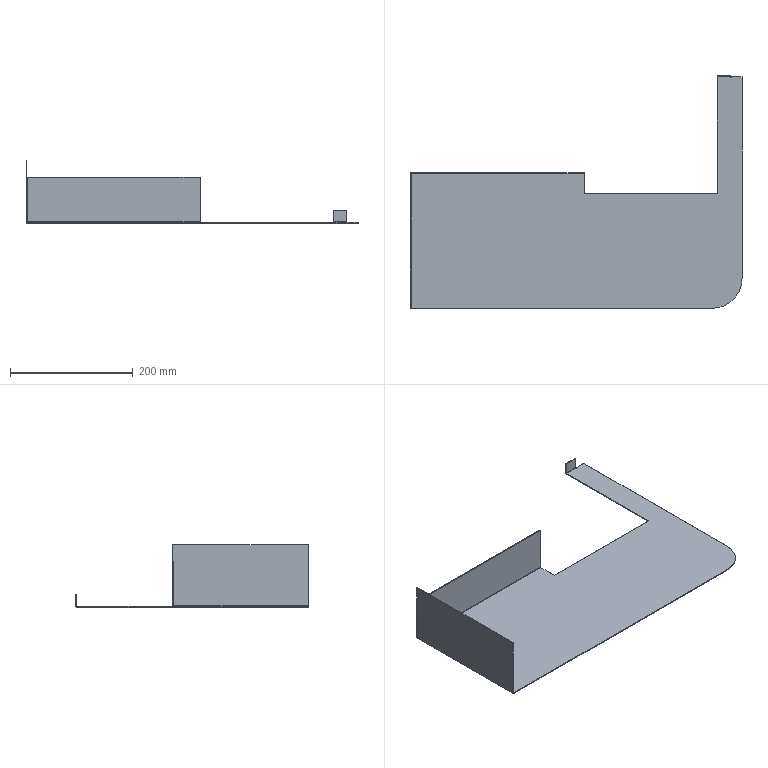Part | SolidWorks | features EdgeFlange 2, FlatPattern 1, SMBaseFlange 1, SMMiteredFlange 1, SheetMetal 1 | 1 solid | 40 faces | box 540.3 x 378.5 x 101.5 mm | volume 241079 mm3 | plane 33 | cylinder 7 | commonest cylinder face diameters 1 x3 4 x3 96.6 x1
STEP:
#1=CARTESIAN_POINT('',(439.153,446.521,-1.5));
#2=VERTEX_POINT('',#1);
#3=CARTESIAN_POINT('',(417.653,446.521,-1.5));
#4=VERTEX_POINT('',#3);
#5=CARTESIAN_POINT('',(657.653,446.521,-1.5));
#6=DIRECTION('',(-1.,0.,0.));
#7=VECTOR('',#6,1000.);
#8=LINE('',#5,#7);
#9=EDGE_CURVE('',#2,#4,#8,.T.);
#10=ORIENTED_EDGE('',*,*,#9,.F.);
#11=CARTESIAN_POINT('',(439.153,445.771,-1.5));
#12=VERTEX_POINT('',#11);
#13=CARTESIAN_POINT('',(439.153,447.021,-1.5));
#14=DIRECTION('',(0.,-1.,0.));
#15=VECTOR('',#14,1000.);
#16=LINE('',#13,#15);
#17=EDGE_CURVE('',#2,#12,#16,.T.);
#18=ORIENTED_EDGE('',*,*,#17,.T.);
#19=CARTESIAN_POINT('',(439.903,445.771,-1.5));
#20=VERTEX_POINT('',#19);
#21=CARTESIAN_POINT('',(439.153,445.771,-1.5));
#22=DIRECTION('',(1.,0.,0.));
#23=VECTOR('',#22,1000.);
#24=LINE('',#21,#23);
#25=EDGE_CURVE('',#12,#20,#24,.T.);
#26=ORIENTED_EDGE('',*,*,#25,.T.);
#27=CARTESIAN_POINT('',(439.903,447.021,-1.5));
#28=VERTEX_POINT('',#27);
#29=CARTESIAN_POINT('',(439.903,445.771,-1.5));
#30=DIRECTION('',(0.,1.,0.));
#31=VECTOR('',#30,1000.);
#32=LINE('',#29,#31);
#33=EDGE_CURVE('',#20,#28,#32,.T.);
#34=ORIENTED_EDGE('',*,*,#33,.T.);
#35=CARTESIAN_POINT('',(457.653,447.021,-1.5));
#36=VERTEX_POINT('',#35);
#37=CARTESIAN_POINT('',(417.653,447.021,-1.5));
#38=DIRECTION('',(-1.,0.,0.));
#39=VECTOR('',#38,1000.);
#40=LINE('',#37,#39);
#41=EDGE_CURVE('',#36,#28,#40,.T.);
#42=ORIENTED_EDGE('',*,*,#41,.F.);
#43=CARTESIAN_POINT('',(457.653,118.321,-1.5));
#44=VERTEX_POINT('',#43);
#45=CARTESIAN_POINT('',(457.653,118.321,-1.5));
#46=DIRECTION('',(0.,1.,0.));
#47=VECTOR('',#46,1000.);
#48=LINE('',#45,#47);
#49=EDGE_CURVE('',#44,#36,#48,.T.);
#50=ORIENTED_EDGE('',*,*,#49,.F.);
#51=CARTESIAN_POINT('',(409.353,70.021,-1.5));
#52=VERTEX_POINT('',#51);
#53=CARTESIAN_POINT('',(409.353,118.321,-1.5));
#54=DIRECTION('',(0.,0.,1.));
#55=DIRECTION('',(1.,0.,0.));
#56=AXIS2_PLACEMENT_3D('',#53,#54,#55);
#57=CIRCLE('',#56,48.3);
#58=EDGE_CURVE('',#52,#44,#57,.T.);
#59=ORIENTED_EDGE('',*,*,#58,.F.);
#60=CARTESIAN_POINT('',(-80.647,70.021,-1.5));
#61=VERTEX_POINT('',#60);
#62=CARTESIAN_POINT('',(-82.647,70.021,-1.5));
#63=DIRECTION('',(1.,0.,0.));
#64=VECTOR('',#63,1000.);
#65=LINE('',#62,#64);
#66=EDGE_CURVE('',#61,#52,#65,.T.);
#67=ORIENTED_EDGE('',*,*,#66,.F.);
#68=CARTESIAN_POINT('',(-80.647,288.821,-1.5));
#69=VERTEX_POINT('',#68);
#70=CARTESIAN_POINT('',(-80.647,70.021,-1.5));
#71=DIRECTION('',(0.,1.,0.));
#72=VECTOR('',#71,1000.);
#73=LINE('',#70,#72);
#74=EDGE_CURVE('',#61,#69,#73,.T.);
#75=ORIENTED_EDGE('',*,*,#74,.T.);
#76=CARTESIAN_POINT('',(200.653,288.821,-1.5));
#77=VERTEX_POINT('',#76);
#78=CARTESIAN_POINT('',(-80.647,288.821,-1.5));
#79=DIRECTION('',(1.,0.,0.));
#80=VECTOR('',#79,1000.);
#81=LINE('',#78,#80);
#82=EDGE_CURVE('',#69,#77,#81,.T.);
#83=ORIENTED_EDGE('',*,*,#82,.T.);
#84=CARTESIAN_POINT('',(200.653,257.521,-1.5));
#85=VERTEX_POINT('',#84);
#86=CARTESIAN_POINT('',(200.653,257.521,-1.5));
#87=DIRECTION('',(0.,1.,0.));
#88=VECTOR('',#87,1000.);
#89=LINE('',#86,#88);
#90=EDGE_CURVE('',#85,#77,#89,.T.);
#91=ORIENTED_EDGE('',*,*,#90,.F.);
#92=CARTESIAN_POINT('',(417.653,257.521,-1.5));
#93=VERTEX_POINT('',#92);
#94=CARTESIAN_POINT('',(417.653,257.521,-1.5));
#95=DIRECTION('',(-1.,0.,0.));
#96=VECTOR('',#95,1000.);
#97=LINE('',#94,#96);
#98=EDGE_CURVE('',#93,#85,#97,.T.);
#99=ORIENTED_EDGE('',*,*,#98,.F.);
#100=CARTESIAN_POINT('',(417.653,447.021,-1.5));
#101=DIRECTION('',(0.,-1.,0.));
#102=VECTOR('',#101,1000.);
#103=LINE('',#100,#102);
#104=EDGE_CURVE('',#4,#93,#103,.T.);
#105=ORIENTED_EDGE('',*,*,#104,.F.);
#106=EDGE_LOOP('',(#10,#18,#26,#34,#42,#50,#59,#67,#75,#83,#91,#99,#105));
#107=FACE_OUTER_BOUND('',#106,.T.);
#108=CARTESIAN_POINT('',(409.353,118.321,-1.5));
#109=DIRECTION('',(0.,0.,1.));
#110=DIRECTION('',(1.,0.,0.));
#111=AXIS2_PLACEMENT_3D('',#108,#109,#110);
#112=PLANE('',#111);
#113=ADVANCED_FACE('',(#107),#112,.F.);
#114=CARTESIAN_POINT('',(439.153,446.521,0.));
#115=VERTEX_POINT('',#114);
#116=CARTESIAN_POINT('',(439.153,445.771,0.));
#117=VERTEX_POINT('',#116);
#118=CARTESIAN_POINT('',(439.153,447.021,0.));
#119=DIRECTION('',(0.,-1.,0.));
#120=VECTOR('',#119,1000.);
#121=LINE('',#118,#120);
#122=EDGE_CURVE('',#115,#117,#121,.T.);
#123=ORIENTED_EDGE('',*,*,#122,.F.);
#124=CARTESIAN_POINT('',(417.653,446.521,0.));
#125=VERTEX_POINT('',#124);
#126=CARTESIAN_POINT('',(657.653,446.521,0.));
#127=DIRECTION('',(-1.,0.,0.));
#128=VECTOR('',#127,1000.);
#129=LINE('',#126,#128);
#130=EDGE_CURVE('',#115,#125,#129,.T.);
#131=ORIENTED_EDGE('',*,*,#130,.T.);
#132=CARTESIAN_POINT('',(417.653,257.521,0.));
#133=VERTEX_POINT('',#132);
#134=CARTESIAN_POINT('',(417.653,447.021,0.));
#135=DIRECTION('',(0.,-1.,0.));
#136=VECTOR('',#135,1000.);
#137=LINE('',#134,#136);
#138=EDGE_CURVE('',#125,#133,#137,.T.);
#139=ORIENTED_EDGE('',*,*,#138,.T.);
#140=CARTESIAN_POINT('',(200.653,257.521,0.));
#141=VERTEX_POINT('',#140);
#142=CARTESIAN_POINT('',(417.653,257.521,0.));
#143=DIRECTION('',(-1.,0.,0.));
#144=VECTOR('',#143,1000.);
#145=LINE('',#142,#144);
#146=EDGE_CURVE('',#133,#141,#145,.T.);
#147=ORIENTED_EDGE('',*,*,#146,.T.);
#148=CARTESIAN_POINT('',(200.653,288.821,0.));
#149=VERTEX_POINT('',#148);
#150=CARTESIAN_POINT('',(200.653,257.521,0.));
#151=DIRECTION('',(0.,1.,0.));
#152=VECTOR('',#151,1000.);
#153=LINE('',#150,#152);
#154=EDGE_CURVE('',#141,#149,#153,.T.);
#155=ORIENTED_EDGE('',*,*,#154,.T.);
#156=CARTESIAN_POINT('',(-80.647,288.821,0.));
#157=VERTEX_POINT('',#156);
#158=CARTESIAN_POINT('',(-80.647,288.821,0.));
#159=DIRECTION('',(1.,0.,0.));
#160=VECTOR('',#159,1000.);
#161=LINE('',#158,#160);
#162=EDGE_CURVE('',#157,#149,#161,.T.);
#163=ORIENTED_EDGE('',*,*,#162,.F.);
#164=CARTESIAN_POINT('',(-80.647,70.021,0.));
#165=VERTEX_POINT('',#164);
#166=CARTESIAN_POINT('',(-80.647,70.021,0.));
#167=DIRECTION('',(0.,1.,0.));
#168=VECTOR('',#167,1000.);
#169=LINE('',#166,#168);
#170=EDGE_CURVE('',#165,#157,#169,.T.);
#171=ORIENTED_EDGE('',*,*,#170,.F.);
#172=CARTESIAN_POINT('',(409.353,70.021,0.));
#173=VERTEX_POINT('',#172);
#174=CARTESIAN_POINT('',(-82.647,70.021,0.));
#175=DIRECTION('',(1.,0.,0.));
#176=VECTOR('',#175,1000.);
#177=LINE('',#174,#176);
#178=EDGE_CURVE('',#165,#173,#177,.T.);
#179=ORIENTED_EDGE('',*,*,#178,.T.);
#180=CARTESIAN_POINT('',(457.653,118.321,0.));
#181=VERTEX_POINT('',#180);
#182=CARTESIAN_POINT('',(409.353,118.321,0.));
#183=DIRECTION('',(0.,0.,1.));
#184=DIRECTION('',(1.,0.,0.));
#185=AXIS2_PLACEMENT_3D('',#182,#183,#184);
#186=CIRCLE('',#185,48.3);
#187=EDGE_CURVE('',#173,#181,#186,.T.);
#188=ORIENTED_EDGE('',*,*,#187,.T.);
#189=CARTESIAN_POINT('',(457.653,447.021,0.));
#190=VERTEX_POINT('',#189);
#191=CARTESIAN_POINT('',(457.653,118.321,0.));
#192=DIRECTION('',(0.,1.,0.));
#193=VECTOR('',#192,1000.);
#194=LINE('',#191,#193);
#195=EDGE_CURVE('',#181,#190,#194,.T.);
#196=ORIENTED_EDGE('',*,*,#195,.T.);
#197=CARTESIAN_POINT('',(439.903,447.021,0.));
#198=VERTEX_POINT('',#197);
#199=CARTESIAN_POINT('',(417.653,447.021,0.));
#200=DIRECTION('',(-1.,0.,0.));
#201=VECTOR('',#200,1000.);
#202=LINE('',#199,#201);
#203=EDGE_CURVE('',#190,#198,#202,.T.);
#204=ORIENTED_EDGE('',*,*,#203,.T.);
#205=CARTESIAN_POINT('',(439.903,445.771,0.));
#206=VERTEX_POINT('',#205);
#207=CARTESIAN_POINT('',(439.903,445.771,0.));
#208=DIRECTION('',(0.,1.,0.));
#209=VECTOR('',#208,1000.);
#210=LINE('',#207,#209);
#211=EDGE_CURVE('',#206,#198,#210,.T.);
#212=ORIENTED_EDGE('',*,*,#211,.F.);
#213=CARTESIAN_POINT('',(439.153,445.771,0.));
#214=DIRECTION('',(1.,0.,0.));
#215=VECTOR('',#214,1000.);
#216=LINE('',#213,#215);
#217=EDGE_CURVE('',#117,#206,#216,.T.);
#218=ORIENTED_EDGE('',*,*,#217,.F.);
#219=EDGE_LOOP('',(#123,#131,#139,#147,#155,#163,#171,#179,#188,#196,#204,#212,#218));
#220=FACE_OUTER_BOUND('',#219,.T.);
#221=CARTESIAN_POINT('',(409.353,118.321,0.));
#222=DIRECTION('',(0.,0.,1.));
#223=DIRECTION('',(1.,0.,0.));
#224=AXIS2_PLACEMENT_3D('',#221,#222,#223);
#225=PLANE('',#224);
#226=ADVANCED_FACE('',(#220),#225,.T.);
#227=ORIENTED_EDGE('',*,*,#138,.F.);
#228=CARTESIAN_POINT('',(417.653,446.521,0.));
#229=DIRECTION('',(0.,0.,-1.));
#230=VECTOR('',#229,1000.);
#231=LINE('',#228,#230);
#232=EDGE_CURVE('',#125,#4,#231,.T.);
#233=ORIENTED_EDGE('',*,*,#232,.T.);
#234=ORIENTED_EDGE('',*,*,#104,.T.);
#235=CARTESIAN_POINT('',(417.653,257.521,-1.5));
#236=DIRECTION('',(0.,0.,1.));
#237=VECTOR('',#236,1000.);
#238=LINE('',#235,#237);
#239=EDGE_CURVE('',#93,#133,#238,.T.);
#240=ORIENTED_EDGE('',*,*,#239,.T.);
#241=EDGE_LOOP('',(#227,#233,#234,#240));
#242=FACE_OUTER_BOUND('',#241,.T.);
#243=CARTESIAN_POINT('',(417.653,447.021,-1.5));
#244=DIRECTION('',(-1.,0.,0.));
#245=DIRECTION('',(0.,-1.,0.));
#246=AXIS2_PLACEMENT_3D('',#243,#244,#245);
#247=PLANE('',#246);
#248=ADVANCED_FACE('',(#242),#247,.T.);
#249=ORIENTED_EDGE('',*,*,#41,.T.);
#250=CARTESIAN_POINT('',(439.903,447.021,0.));
#251=DIRECTION('',(0.,0.,-1.));
#252=VECTOR('',#251,1000.);
#253=LINE('',#250,#252);
#254=EDGE_CURVE('',#198,#28,#253,.T.);
#255=ORIENTED_EDGE('',*,*,#254,.F.);
#256=ORIENTED_EDGE('',*,*,#203,.F.);
#257=CARTESIAN_POINT('',(457.653,447.021,-1.5));
#258=DIRECTION('',(0.,0.,1.));
#259=VECTOR('',#258,1000.);
#260=LINE('',#257,#259);
#261=EDGE_CURVE('',#36,#190,#260,.T.);
#262=ORIENTED_EDGE('',*,*,#261,.F.);
#263=EDGE_LOOP('',(#249,#255,#256,#262));
#264=FACE_OUTER_BOUND('',#263,.T.);
#265=CARTESIAN_POINT('',(417.653,447.021,-1.5));
#266=DIRECTION('',(0.,1.,0.));
#267=DIRECTION('',(-1.,0.,0.));
#268=AXIS2_PLACEMENT_3D('',#265,#266,#267);
#269=PLANE('',#268);
#270=ADVANCED_FACE('',(#264),#269,.T.);
#271=CARTESIAN_POINT('',(-82.647,288.821,0.5));
#272=VERTEX_POINT('',#271);
#273=CARTESIAN_POINT('',(-81.147,288.821,0.5));
#274=VERTEX_POINT('',#273);
#275=CARTESIAN_POINT('',(-82.647,288.821,0.5));
#276=DIRECTION('',(1.,0.,0.));
#277=VECTOR('',#276,1000.);
#278=LINE('',#275,#277);
#279=EDGE_CURVE('',#272,#274,#278,.T.);
#280=ORIENTED_EDGE('',*,*,#279,.F.);
#281=CARTESIAN_POINT('',(-82.647,290.821,0.5));
#282=VERTEX_POINT('',#281);
#283=CARTESIAN_POINT('',(-82.647,0.,0.5));
#284=DIRECTION('',(0.,-1.,0.));
#285=VECTOR('',#284,1000.);
#286=LINE('',#283,#285);
#287=EDGE_CURVE('',#282,#272,#286,.T.);
#288=ORIENTED_EDGE('',*,*,#287,.F.);
#289=CARTESIAN_POINT('',(-81.147,290.821,0.5));
#290=VERTEX_POINT('',#289);
#291=CARTESIAN_POINT('',(-82.647,290.821,0.5));
#292=DIRECTION('',(-1.,0.,0.));
#293=VECTOR('',#292,1000.);
#294=LINE('',#291,#293);
#295=EDGE_CURVE('',#290,#282,#294,.T.);
#296=ORIENTED_EDGE('',*,*,#295,.F.);
#297=CARTESIAN_POINT('',(-81.147,290.821,0.5));
#298=DIRECTION('',(0.,-1.,0.));
#299=VECTOR('',#298,1000.);
#300=LINE('',#297,#299);
#301=EDGE_CURVE('',#290,#274,#300,.T.);
#302=ORIENTED_EDGE('',*,*,#301,.T.);
#303=EDGE_LOOP('',(#280,#288,#296,#302));
#304=FACE_OUTER_BOUND('',#303,.T.);
#305=CARTESIAN_POINT('',(0.,0.,0.5));
#306=DIRECTION('',(0.,0.,-1.));
#307=DIRECTION('',(-1.,0.,0.));
#308=AXIS2_PLACEMENT_3D('',#305,#306,#307);
#309=PLANE('',#308);
#310=ADVANCED_FACE('',(#304),#309,.T.);
#311=CARTESIAN_POINT('',(-82.647,70.021,0.5));
#312=VERTEX_POINT('',#311);
#313=CARTESIAN_POINT('',(-82.647,0.,0.5));
#314=DIRECTION('',(0.,-1.,0.));
#315=VECTOR('',#314,1000.);
#316=LINE('',#313,#315);
#317=EDGE_CURVE('',#272,#312,#316,.T.);
#318=ORIENTED_EDGE('',*,*,#317,.F.);
#319=CARTESIAN_POINT('',(-80.647,288.821,0.5));
#320=DIRECTION('',(0.,-1.,0.));
#321=DIRECTION('',(0.,0.,1.));
#322=AXIS2_PLACEMENT_3D('',#319,#320,#321);
#323=CIRCLE('',#322,2.);
#324=EDGE_CURVE('',#272,#69,#323,.T.);
#325=ORIENTED_EDGE('',*,*,#324,.T.);
#326=ORIENTED_EDGE('',*,*,#74,.F.);
#327=CARTESIAN_POINT('',(-80.647,70.021,0.5));
#328=DIRECTION('',(0.,-1.,0.));
#329=DIRECTION('',(0.,0.,-1.));
#330=AXIS2_PLACEMENT_3D('',#327,#328,#329);
#331=CIRCLE('',#330,2.);
#332=EDGE_CURVE('',#312,#61,#331,.T.);
#333=ORIENTED_EDGE('',*,*,#332,.F.);
#334=EDGE_LOOP('',(#318,#325,#326,#333));
#335=FACE_OUTER_BOUND('',#334,.T.);
#336=CARTESIAN_POINT('',(-80.647,70.021,0.5));
#337=DIRECTION('',(0.,-1.,0.));
#338=DIRECTION('',(-1.,0.,0.));
#339=AXIS2_PLACEMENT_3D('',#336,#337,#338);
#340=CYLINDRICAL_SURFACE('',#339,2.);
#341=ADVANCED_FACE('',(#335),#340,.T.);
#342=ORIENTED_EDGE('',*,*,#178,.F.);
#343=CARTESIAN_POINT('',(-80.647,70.021,0.));
#344=DIRECTION('',(0.,0.,-1.));
#345=VECTOR('',#344,1000.);
#346=LINE('',#343,#345);
#347=EDGE_CURVE('',#165,#61,#346,.T.);
#348=ORIENTED_EDGE('',*,*,#347,.T.);
#349=ORIENTED_EDGE('',*,*,#66,.T.);
#350=CARTESIAN_POINT('',(409.353,70.021,-1.5));
#351=DIRECTION('',(0.,0.,1.));
#352=VECTOR('',#351,1000.);
#353=LINE('',#350,#352);
#354=EDGE_CURVE('',#52,#173,#353,.T.);
#355=ORIENTED_EDGE('',*,*,#354,.T.);
#356=EDGE_LOOP('',(#342,#348,#349,#355));
#357=FACE_OUTER_BOUND('',#356,.T.);
#358=CARTESIAN_POINT('',(-82.647,70.021,-1.5));
#359=DIRECTION('',(0.,-1.,0.));
#360=DIRECTION('',(1.,0.,0.));
#361=AXIS2_PLACEMENT_3D('',#358,#359,#360);
#362=PLANE('',#361);
#363=ADVANCED_FACE('',(#357),#362,.T.);
#364=CARTESIAN_POINT('',(200.653,288.821,0.));
#365=DIRECTION('',(0.,0.,-1.));
#366=VECTOR('',#365,1000.);
#367=LINE('',#364,#366);
#368=EDGE_CURVE('',#149,#77,#367,.T.);
#369=ORIENTED_EDGE('',*,*,#368,.F.);
#370=ORIENTED_EDGE('',*,*,#154,.F.);
#371=CARTESIAN_POINT('',(200.653,257.521,-1.5));
#372=DIRECTION('',(0.,0.,1.));
#373=VECTOR('',#372,1000.);
#374=LINE('',#371,#373);
#375=EDGE_CURVE('',#85,#141,#374,.T.);
#376=ORIENTED_EDGE('',*,*,#375,.F.);
#377=ORIENTED_EDGE('',*,*,#90,.T.);
#378=EDGE_LOOP('',(#369,#370,#376,#377));
#379=FACE_OUTER_BOUND('',#378,.T.);
#380=CARTESIAN_POINT('',(200.653,257.521,-1.5));
#381=DIRECTION('',(1.,0.,0.));
#382=DIRECTION('',(0.,1.,0.));
#383=AXIS2_PLACEMENT_3D('',#380,#381,#382);
#384=PLANE('',#383);
#385=ADVANCED_FACE('',(#379),#384,.T.);
#386=ORIENTED_EDGE('',*,*,#146,.F.);
#387=ORIENTED_EDGE('',*,*,#239,.F.);
#388=ORIENTED_EDGE('',*,*,#98,.T.);
#389=ORIENTED_EDGE('',*,*,#375,.T.);
#390=EDGE_LOOP('',(#386,#387,#388,#389));
#391=FACE_OUTER_BOUND('',#390,.T.);
#392=CARTESIAN_POINT('',(417.653,257.521,-1.5));
#393=DIRECTION('',(0.,1.,0.));
#394=DIRECTION('',(-1.,0.,0.));
#395=AXIS2_PLACEMENT_3D('',#392,#393,#394);
#396=PLANE('',#395);
#397=ADVANCED_FACE('',(#391),#396,.T.);
#398=ORIENTED_EDGE('',*,*,#195,.F.);
#399=CARTESIAN_POINT('',(457.653,118.321,-1.5));
#400=DIRECTION('',(0.,0.,1.));
#401=VECTOR('',#400,1000.);
#402=LINE('',#399,#401);
#403=EDGE_CURVE('',#44,#181,#402,.T.);
#404=ORIENTED_EDGE('',*,*,#403,.F.);
#405=ORIENTED_EDGE('',*,*,#49,.T.);
#406=ORIENTED_EDGE('',*,*,#261,.T.);
#407=EDGE_LOOP('',(#398,#404,#405,#406));
#408=FACE_OUTER_BOUND('',#407,.T.);
#409=CARTESIAN_POINT('',(457.653,118.321,-1.5));
#410=DIRECTION('',(1.,0.,0.));
#411=DIRECTION('',(0.,1.,0.));
#412=AXIS2_PLACEMENT_3D('',#409,#410,#411);
#413=PLANE('',#412);
#414=ADVANCED_FACE('',(#408),#413,.T.);
#415=ORIENTED_EDGE('',*,*,#187,.F.);
#416=ORIENTED_EDGE('',*,*,#354,.F.);
#417=ORIENTED_EDGE('',*,*,#58,.T.);
#418=ORIENTED_EDGE('',*,*,#403,.T.);
#419=EDGE_LOOP('',(#415,#416,#417,#418));
#420=FACE_OUTER_BOUND('',#419,.T.);
#421=CARTESIAN_POINT('',(409.353,118.321,-1.5));
#422=DIRECTION('',(0.,0.,1.));
#423=DIRECTION('',(1.,0.,0.));
#424=AXIS2_PLACEMENT_3D('',#421,#422,#423);
#425=CYLINDRICAL_SURFACE('',#424,48.3);
#426=ADVANCED_FACE('',(#420),#425,.T.);
#427=CARTESIAN_POINT('',(-81.147,70.021,0.5));
#428=VERTEX_POINT('',#427);
#429=CARTESIAN_POINT('',(-80.647,70.021,0.5));
#430=DIRECTION('',(0.,-1.,0.));
#431=DIRECTION('',(0.,0.,-1.));
#432=AXIS2_PLACEMENT_3D('',#429,#430,#431);
#433=CIRCLE('',#432,0.5);
#434=EDGE_CURVE('',#428,#165,#433,.T.);
#435=ORIENTED_EDGE('',*,*,#434,.F.);
#436=CARTESIAN_POINT('',(-81.147,70.021,0.5));
#437=DIRECTION('',(-1.,0.,0.));
#438=VECTOR('',#437,1000.);
#439=LINE('',#436,#438);
#440=EDGE_CURVE('',#428,#312,#439,.T.);
#441=ORIENTED_EDGE('',*,*,#440,.T.);
#442=ORIENTED_EDGE('',*,*,#332,.T.);
#443=ORIENTED_EDGE('',*,*,#347,.F.);
#444=EDGE_LOOP('',(#435,#441,#442,#443));
#445=FACE_OUTER_BOUND('',#444,.T.);
#446=CARTESIAN_POINT('',(-80.647,70.021,0.5));
#447=DIRECTION('',(0.,1.,0.));
#448=DIRECTION('',(0.,0.,1.));
#449=AXIS2_PLACEMENT_3D('',#446,#447,#448);
#450=PLANE('',#449);
#451=ADVANCED_FACE('',(#445),#450,.F.);
#452=ORIENTED_EDGE('',*,*,#324,.F.);
#453=ORIENTED_EDGE('',*,*,#279,.T.);
#454=CARTESIAN_POINT('',(-80.647,288.821,0.5));
#455=DIRECTION('',(0.,-1.,0.));
#456=DIRECTION('',(0.,0.,1.));
#457=AXIS2_PLACEMENT_3D('',#454,#455,#456);
#458=CIRCLE('',#457,0.5);
#459=EDGE_CURVE('',#274,#157,#458,.T.);
#460=ORIENTED_EDGE('',*,*,#459,.T.);
#461=CARTESIAN_POINT('',(-80.647,288.821,0.));
#462=DIRECTION('',(0.,0.,-1.));
#463=VECTOR('',#462,1000.);
#464=LINE('',#461,#463);
#465=EDGE_CURVE('',#157,#69,#464,.T.);
#466=ORIENTED_EDGE('',*,*,#465,.T.);
#467=EDGE_LOOP('',(#452,#453,#460,#466));
#468=FACE_OUTER_BOUND('',#467,.T.);
#469=CARTESIAN_POINT('',(-80.647,288.821,0.5));
#470=DIRECTION('',(0.,1.,0.));
#471=DIRECTION('',(0.,0.,1.));
#472=AXIS2_PLACEMENT_3D('',#469,#470,#471);
#473=PLANE('',#472);
#474=ADVANCED_FACE('',(#468),#473,.T.);
#475=ORIENTED_EDGE('',*,*,#459,.F.);
#476=CARTESIAN_POINT('',(-81.147,290.821,0.5));
#477=DIRECTION('',(0.,-1.,0.));
#478=VECTOR('',#477,1000.);
#479=LINE('',#476,#478);
#480=EDGE_CURVE('',#274,#428,#479,.T.);
#481=ORIENTED_EDGE('',*,*,#480,.T.);
#482=ORIENTED_EDGE('',*,*,#434,.T.);
#483=ORIENTED_EDGE('',*,*,#170,.T.);
#484=EDGE_LOOP('',(#475,#481,#482,#483));
#485=FACE_OUTER_BOUND('',#484,.T.);
#486=CARTESIAN_POINT('',(-80.647,70.021,0.5));
#487=DIRECTION('',(0.,-1.,0.));
#488=DIRECTION('',(-1.,0.,0.));
#489=AXIS2_PLACEMENT_3D('',#486,#487,#488);
#490=CYLINDRICAL_SURFACE('',#489,0.5);
#491=ADVANCED_FACE('',(#485),#490,.F.);
#492=CARTESIAN_POINT('',(-82.647,70.021,100.));
#493=VERTEX_POINT('',#492);
#494=CARTESIAN_POINT('',(-82.647,70.021,0.));
#495=DIRECTION('',(0.,0.,-1.));
#496=VECTOR('',#495,1000.);
#497=LINE('',#494,#496);
#498=EDGE_CURVE('',#493,#312,#497,.T.);
#499=ORIENTED_EDGE('',*,*,#498,.T.);
#500=ORIENTED_EDGE('',*,*,#440,.F.);
#501=CARTESIAN_POINT('',(-81.147,70.021,100.));
#502=VERTEX_POINT('',#501);
#503=CARTESIAN_POINT('',(-81.147,70.021,0.));
#504=DIRECTION('',(0.,0.,-1.));
#505=VECTOR('',#504,1000.);
#506=LINE('',#503,#505);
#507=EDGE_CURVE('',#502,#428,#506,.T.);
#508=ORIENTED_EDGE('',*,*,#507,.F.);
#509=CARTESIAN_POINT('',(-82.647,70.021,100.));
#510=DIRECTION('',(1.,0.,0.));
#511=VECTOR('',#510,1000.);
#512=LINE('',#509,#511);
#513=EDGE_CURVE('',#493,#502,#512,.T.);
#514=ORIENTED_EDGE('',*,*,#513,.F.);
#515=EDGE_LOOP('',(#499,#500,#508,#514));
#516=FACE_OUTER_BOUND('',#515,.T.);
#517=CARTESIAN_POINT('',(-82.647,70.021,0.));
#518=DIRECTION('',(0.,-1.,0.));
#519=DIRECTION('',(1.,0.,0.));
#520=AXIS2_PLACEMENT_3D('',#517,#518,#519);
#521=PLANE('',#520);
#522=ADVANCED_FACE('',(#516),#521,.T.);
#523=CARTESIAN_POINT('',(-81.147,290.821,100.));
#524=VERTEX_POINT('',#523);
#525=CARTESIAN_POINT('',(-81.147,290.821,0.));
#526=DIRECTION('',(0.,0.,1.));
#527=VECTOR('',#526,1000.);
#528=LINE('',#525,#527);
#529=EDGE_CURVE('',#290,#524,#528,.T.);
#530=ORIENTED_EDGE('',*,*,#529,.F.);
#531=ORIENTED_EDGE('',*,*,#295,.T.);
#532=CARTESIAN_POINT('',(-82.647,290.821,100.));
#533=VERTEX_POINT('',#532);
#534=CARTESIAN_POINT('',(-82.647,290.821,100.));
#535=DIRECTION('',(0.,0.,1.));
#536=VECTOR('',#535,1000.);
#537=LINE('',#534,#536);
#538=EDGE_CURVE('',#282,#533,#537,.T.);
#539=ORIENTED_EDGE('',*,*,#538,.T.);
#540=CARTESIAN_POINT('',(-82.647,290.821,100.));
#541=DIRECTION('',(1.,0.,0.));
#542=VECTOR('',#541,1000.);
#543=LINE('',#540,#542);
#544=EDGE_CURVE('',#533,#524,#543,.T.);
#545=ORIENTED_EDGE('',*,*,#544,.T.);
#546=EDGE_LOOP('',(#530,#531,#539,#545));
#547=FACE_OUTER_BOUND('',#546,.T.);
#548=CARTESIAN_POINT('',(-82.647,290.821,100.));
#549=DIRECTION('',(0.,1.,0.));
#550=DIRECTION('',(-1.,0.,0.));
#551=AXIS2_PLACEMENT_3D('',#548,#549,#550);
#552=PLANE('',#551);
#553=ADVANCED_FACE('',(#547),#552,.T.);
#554=ORIENTED_EDGE('',*,*,#538,.F.);
#555=ORIENTED_EDGE('',*,*,#287,.T.);
#556=ORIENTED_EDGE('',*,*,#317,.T.);
#557=ORIENTED_EDGE('',*,*,#498,.F.);
#558=CARTESIAN_POINT('',(-82.647,70.021,100.));
#559=DIRECTION('',(0.,-1.,0.));
#560=VECTOR('',#559,1000.);
#561=LINE('',#558,#560);
#562=EDGE_CURVE('',#533,#493,#561,.T.);
#563=ORIENTED_EDGE('',*,*,#562,.F.);
#564=EDGE_LOOP('',(#554,#555,#556,#557,#563));
#565=FACE_OUTER_BOUND('',#564,.T.);
#566=CARTESIAN_POINT('',(-82.647,0.,0.));
#567=DIRECTION('',(-1.,0.,0.));
#568=DIRECTION('',(0.,0.,1.));
#569=AXIS2_PLACEMENT_3D('',#566,#567,#568);
#570=PLANE('',#569);
#571=ADVANCED_FACE('',(#565),#570,.T.);
#572=ORIENTED_EDGE('',*,*,#301,.F.);
#573=ORIENTED_EDGE('',*,*,#529,.T.);
#574=CARTESIAN_POINT('',(-81.147,0.,100.));
#575=DIRECTION('',(0.,-1.,0.));
#576=VECTOR('',#575,1000.);
#577=LINE('',#574,#576);
#578=EDGE_CURVE('',#524,#502,#577,.T.);
#579=ORIENTED_EDGE('',*,*,#578,.T.);
#580=ORIENTED_EDGE('',*,*,#507,.T.);
#581=ORIENTED_EDGE('',*,*,#480,.F.);
#582=EDGE_LOOP('',(#572,#573,#579,#580,#581));
#583=FACE_OUTER_BOUND('',#582,.T.);
#584=CARTESIAN_POINT('',(-81.147,0.,0.));
#585=DIRECTION('',(-1.,0.,0.));
#586=DIRECTION('',(0.,0.,1.));
#587=AXIS2_PLACEMENT_3D('',#584,#585,#586);
#588=PLANE('',#587);
#589=ADVANCED_FACE('',(#583),#588,.F.);
#590=ORIENTED_EDGE('',*,*,#578,.F.);
#591=ORIENTED_EDGE('',*,*,#544,.F.);
#592=ORIENTED_EDGE('',*,*,#562,.T.);
#593=ORIENTED_EDGE('',*,*,#513,.T.);
#594=EDGE_LOOP('',(#590,#591,#592,#593));
#595=FACE_OUTER_BOUND('',#594,.T.);
#596=CARTESIAN_POINT('',(-82.647,70.021,100.));
#597=DIRECTION('',(0.,0.,1.));
#598=DIRECTION('',(1.,0.,0.));
#599=AXIS2_PLACEMENT_3D('',#596,#597,#598);
#600=PLANE('',#599);
#601=ADVANCED_FACE('',(#595),#600,.T.);
#602=CARTESIAN_POINT('',(200.653,289.321,0.5));
#603=VERTEX_POINT('',#602);
#604=CARTESIAN_POINT('',(200.653,290.821,0.5));
#605=VERTEX_POINT('',#604);
#606=CARTESIAN_POINT('',(200.653,290.821,0.5));
#607=DIRECTION('',(0.,1.,0.));
#608=VECTOR('',#607,1000.);
#609=LINE('',#606,#608);
#610=EDGE_CURVE('',#603,#605,#609,.T.);
#611=ORIENTED_EDGE('',*,*,#610,.F.);
#612=CARTESIAN_POINT('',(200.653,288.821,0.5));
#613=DIRECTION('',(1.,0.,0.));
#614=DIRECTION('',(0.,0.,1.));
#615=AXIS2_PLACEMENT_3D('',#612,#613,#614);
#616=CIRCLE('',#615,0.5);
#617=EDGE_CURVE('',#149,#603,#616,.T.);
#618=ORIENTED_EDGE('',*,*,#617,.F.);
#619=ORIENTED_EDGE('',*,*,#368,.T.);
#620=CARTESIAN_POINT('',(200.653,288.821,0.5));
#621=DIRECTION('',(1.,0.,0.));
#622=DIRECTION('',(0.,0.,1.));
#623=AXIS2_PLACEMENT_3D('',#620,#621,#622);
#624=CIRCLE('',#623,2.);
#625=EDGE_CURVE('',#77,#605,#624,.T.);
#626=ORIENTED_EDGE('',*,*,#625,.T.);
#627=EDGE_LOOP('',(#611,#618,#619,#626));
#628=FACE_OUTER_BOUND('',#627,.T.);
#629=CARTESIAN_POINT('',(200.653,288.821,0.5));
#630=DIRECTION('',(1.,0.,0.));
#631=DIRECTION('',(0.,0.,-1.));
#632=AXIS2_PLACEMENT_3D('',#629,#630,#631);
#633=PLANE('',#632);
#634=ADVANCED_FACE('',(#628),#633,.T.);
#635=CARTESIAN_POINT('',(-80.647,289.321,0.5));
#636=VERTEX_POINT('',#635);
#637=CARTESIAN_POINT('',(-80.647,288.821,0.5));
#638=DIRECTION('',(-1.,0.,0.));
#639=DIRECTION('',(0.,0.,1.));
#640=AXIS2_PLACEMENT_3D('',#637,#638,#639);
#641=CIRCLE('',#640,0.5);
#642=EDGE_CURVE('',#636,#157,#641,.T.);
#643=ORIENTED_EDGE('',*,*,#642,.F.);
#644=CARTESIAN_POINT('',(-80.647,290.821,0.5));
#645=VERTEX_POINT('',#644);
#646=CARTESIAN_POINT('',(-80.647,289.321,0.5));
#647=DIRECTION('',(0.,1.,0.));
#648=VECTOR('',#647,1000.);
#649=LINE('',#646,#648);
#650=EDGE_CURVE('',#636,#645,#649,.T.);
#651=ORIENTED_EDGE('',*,*,#650,.T.);
#652=CARTESIAN_POINT('',(-80.647,288.821,0.5));
#653=DIRECTION('',(-1.,0.,0.));
#654=DIRECTION('',(0.,0.,1.));
#655=AXIS2_PLACEMENT_3D('',#652,#653,#654);
#656=CIRCLE('',#655,2.);
#657=EDGE_CURVE('',#645,#69,#656,.T.);
#658=ORIENTED_EDGE('',*,*,#657,.T.);
#659=ORIENTED_EDGE('',*,*,#465,.F.);
#660=EDGE_LOOP('',(#643,#651,#658,#659));
#661=FACE_OUTER_BOUND('',#660,.T.);
#662=CARTESIAN_POINT('',(-80.647,288.821,0.5));
#663=DIRECTION('',(1.,0.,0.));
#664=DIRECTION('',(0.,0.,-1.));
#665=AXIS2_PLACEMENT_3D('',#662,#663,#664);
#666=PLANE('',#665);
#667=ADVANCED_FACE('',(#661),#666,.F.);
#668=ORIENTED_EDGE('',*,*,#82,.F.);
#669=ORIENTED_EDGE('',*,*,#657,.F.);
#670=CARTESIAN_POINT('',(0.,290.821,0.5));
#671=DIRECTION('',(-1.,0.,0.));
#672=VECTOR('',#671,1000.);
#673=LINE('',#670,#672);
#674=EDGE_CURVE('',#605,#645,#673,.T.);
#675=ORIENTED_EDGE('',*,*,#674,.F.);
#676=ORIENTED_EDGE('',*,*,#625,.F.);
#677=EDGE_LOOP('',(#668,#669,#675,#676));
#678=FACE_OUTER_BOUND('',#677,.T.);
#679=CARTESIAN_POINT('',(-80.647,288.821,0.5));
#680=DIRECTION('',(-1.,0.,0.));
#681=DIRECTION('',(0.,1.,0.));
#682=AXIS2_PLACEMENT_3D('',#679,#680,#681);
#683=CYLINDRICAL_SURFACE('',#682,2.);
#684=ADVANCED_FACE('',(#678),#683,.T.);
#685=ORIENTED_EDGE('',*,*,#162,.T.);
#686=ORIENTED_EDGE('',*,*,#617,.T.);
#687=CARTESIAN_POINT('',(200.653,289.321,0.5));
#688=DIRECTION('',(-1.,0.,0.));
#689=VECTOR('',#688,1000.);
#690=LINE('',#687,#689);
#691=EDGE_CURVE('',#603,#636,#690,.T.);
#692=ORIENTED_EDGE('',*,*,#691,.T.);
#693=ORIENTED_EDGE('',*,*,#642,.T.);
#694=EDGE_LOOP('',(#685,#686,#692,#693));
#695=FACE_OUTER_BOUND('',#694,.T.);
#696=CARTESIAN_POINT('',(-80.647,288.821,0.5));
#697=DIRECTION('',(-1.,0.,0.));
#698=DIRECTION('',(0.,1.,0.));
#699=AXIS2_PLACEMENT_3D('',#696,#697,#698);
#700=CYLINDRICAL_SURFACE('',#699,0.5);
#701=ADVANCED_FACE('',(#695),#700,.F.);
#702=CARTESIAN_POINT('',(-80.647,290.821,73.5));
#703=VERTEX_POINT('',#702);
#704=CARTESIAN_POINT('',(-80.647,290.821,0.));
#705=DIRECTION('',(0.,0.,-1.));
#706=VECTOR('',#705,1000.);
#707=LINE('',#704,#706);
#708=EDGE_CURVE('',#703,#645,#707,.T.);
#709=ORIENTED_EDGE('',*,*,#708,.T.);
#710=ORIENTED_EDGE('',*,*,#650,.F.);
#711=CARTESIAN_POINT('',(-80.647,289.321,73.5));
#712=VERTEX_POINT('',#711);
#713=CARTESIAN_POINT('',(-80.647,289.321,0.));
#714=DIRECTION('',(0.,0.,-1.));
#715=VECTOR('',#714,1000.);
#716=LINE('',#713,#715);
#717=EDGE_CURVE('',#712,#636,#716,.T.);
#718=ORIENTED_EDGE('',*,*,#717,.F.);
#719=CARTESIAN_POINT('',(-80.647,290.821,73.5));
#720=DIRECTION('',(0.,-1.,0.));
#721=VECTOR('',#720,1000.);
#722=LINE('',#719,#721);
#723=EDGE_CURVE('',#703,#712,#722,.T.);
#724=ORIENTED_EDGE('',*,*,#723,.F.);
#725=EDGE_LOOP('',(#709,#710,#718,#724));
#726=FACE_OUTER_BOUND('',#725,.T.);
#727=CARTESIAN_POINT('',(-80.647,290.821,0.));
#728=DIRECTION('',(-1.,0.,0.));
#729=DIRECTION('',(0.,-1.,0.));
#730=AXIS2_PLACEMENT_3D('',#727,#728,#729);
#731=PLANE('',#730);
#732=ADVANCED_FACE('',(#726),#731,.T.);
#733=CARTESIAN_POINT('',(200.653,289.321,73.5));
#734=VERTEX_POINT('',#733);
#735=CARTESIAN_POINT('',(200.653,289.321,0.));
#736=DIRECTION('',(0.,0.,1.));
#737=VECTOR('',#736,1000.);
#738=LINE('',#735,#737);
#739=EDGE_CURVE('',#603,#734,#738,.T.);
#740=ORIENTED_EDGE('',*,*,#739,.F.);
#741=ORIENTED_EDGE('',*,*,#610,.T.);
#742=CARTESIAN_POINT('',(200.653,290.821,73.5));
#743=VERTEX_POINT('',#742);
#744=CARTESIAN_POINT('',(200.653,290.821,73.5));
#745=DIRECTION('',(0.,0.,1.));
#746=VECTOR('',#745,1000.);
#747=LINE('',#744,#746);
#748=EDGE_CURVE('',#605,#743,#747,.T.);
#749=ORIENTED_EDGE('',*,*,#748,.T.);
#750=CARTESIAN_POINT('',(200.653,290.821,73.5));
#751=DIRECTION('',(0.,-1.,0.));
#752=VECTOR('',#751,1000.);
#753=LINE('',#750,#752);
#754=EDGE_CURVE('',#743,#734,#753,.T.);
#755=ORIENTED_EDGE('',*,*,#754,.T.);
#756=EDGE_LOOP('',(#740,#741,#749,#755));
#757=FACE_OUTER_BOUND('',#756,.T.);
#758=CARTESIAN_POINT('',(200.653,290.821,73.5));
#759=DIRECTION('',(1.,0.,0.));
#760=DIRECTION('',(0.,1.,0.));
#761=AXIS2_PLACEMENT_3D('',#758,#759,#760);
#762=PLANE('',#761);
#763=ADVANCED_FACE('',(#757),#762,.T.);
#764=ORIENTED_EDGE('',*,*,#748,.F.);
#765=ORIENTED_EDGE('',*,*,#674,.T.);
#766=ORIENTED_EDGE('',*,*,#708,.F.);
#767=CARTESIAN_POINT('',(-80.647,290.821,73.5));
#768=DIRECTION('',(-1.,0.,0.));
#769=VECTOR('',#768,1000.);
#770=LINE('',#767,#769);
#771=EDGE_CURVE('',#743,#703,#770,.T.);
#772=ORIENTED_EDGE('',*,*,#771,.F.);
#773=EDGE_LOOP('',(#764,#765,#766,#772));
#774=FACE_OUTER_BOUND('',#773,.T.);
#775=CARTESIAN_POINT('',(0.,290.821,0.));
#776=DIRECTION('',(0.,1.,0.));
#777=DIRECTION('',(0.,0.,1.));
#778=AXIS2_PLACEMENT_3D('',#775,#776,#777);
#779=PLANE('',#778);
#780=ADVANCED_FACE('',(#774),#779,.T.);
#781=ORIENTED_EDGE('',*,*,#691,.F.);
#782=ORIENTED_EDGE('',*,*,#739,.T.);
#783=CARTESIAN_POINT('',(0.,289.321,73.5));
#784=DIRECTION('',(-1.,0.,0.));
#785=VECTOR('',#784,1000.);
#786=LINE('',#783,#785);
#787=EDGE_CURVE('',#734,#712,#786,.T.);
#788=ORIENTED_EDGE('',*,*,#787,.T.);
#789=ORIENTED_EDGE('',*,*,#717,.T.);
#790=EDGE_LOOP('',(#781,#782,#788,#789));
#791=FACE_OUTER_BOUND('',#790,.T.);
#792=CARTESIAN_POINT('',(0.,289.321,0.));
#793=DIRECTION('',(0.,1.,0.));
#794=DIRECTION('',(0.,0.,1.));
#795=AXIS2_PLACEMENT_3D('',#792,#793,#794);
#796=PLANE('',#795);
#797=ADVANCED_FACE('',(#791),#796,.F.);
#798=ORIENTED_EDGE('',*,*,#787,.F.);
#799=ORIENTED_EDGE('',*,*,#754,.F.);
#800=ORIENTED_EDGE('',*,*,#771,.T.);
#801=ORIENTED_EDGE('',*,*,#723,.T.);
#802=EDGE_LOOP('',(#798,#799,#800,#801));
#803=FACE_OUTER_BOUND('',#802,.T.);
#804=CARTESIAN_POINT('',(-80.647,290.821,73.5));
#805=DIRECTION('',(0.,0.,1.));
#806=DIRECTION('',(0.,-1.,0.));
#807=AXIS2_PLACEMENT_3D('',#804,#805,#806);
#808=PLANE('',#807);
#809=ADVANCED_FACE('',(#803),#808,.T.);
#810=ORIENTED_EDGE('',*,*,#122,.T.);
#811=CARTESIAN_POINT('',(439.153,445.771,0.));
#812=DIRECTION('',(0.,0.,-1.));
#813=VECTOR('',#812,1000.);
#814=LINE('',#811,#813);
#815=EDGE_CURVE('',#117,#12,#814,.T.);
#816=ORIENTED_EDGE('',*,*,#815,.T.);
#817=ORIENTED_EDGE('',*,*,#17,.F.);
#818=CARTESIAN_POINT('',(439.153,446.521,0.));
#819=DIRECTION('',(0.,0.,-1.));
#820=VECTOR('',#819,1000.);
#821=LINE('',#818,#820);
#822=EDGE_CURVE('',#115,#2,#821,.T.);
#823=ORIENTED_EDGE('',*,*,#822,.F.);
#824=EDGE_LOOP('',(#810,#816,#817,#823));
#825=FACE_OUTER_BOUND('',#824,.T.);
#826=CARTESIAN_POINT('',(439.153,447.021,0.));
#827=DIRECTION('',(1.,0.,0.));
#828=DIRECTION('',(0.,0.,-1.));
#829=AXIS2_PLACEMENT_3D('',#826,#827,#828);
#830=PLANE('',#829);
#831=ADVANCED_FACE('',(#825),#830,.T.);
#832=ORIENTED_EDGE('',*,*,#25,.F.);
#833=ORIENTED_EDGE('',*,*,#815,.F.);
#834=ORIENTED_EDGE('',*,*,#217,.T.);
#835=CARTESIAN_POINT('',(439.903,445.771,0.));
#836=DIRECTION('',(0.,0.,-1.));
#837=VECTOR('',#836,1000.);
#838=LINE('',#835,#837);
#839=EDGE_CURVE('',#206,#20,#838,.T.);
#840=ORIENTED_EDGE('',*,*,#839,.T.);
#841=EDGE_LOOP('',(#832,#833,#834,#840));
#842=FACE_OUTER_BOUND('',#841,.T.);
#843=CARTESIAN_POINT('',(439.153,445.771,0.));
#844=DIRECTION('',(0.,1.,0.));
#845=DIRECTION('',(0.,0.,1.));
#846=AXIS2_PLACEMENT_3D('',#843,#844,#845);
#847=PLANE('',#846);
#848=ADVANCED_FACE('',(#842),#847,.T.);
#849=ORIENTED_EDGE('',*,*,#33,.F.);
#850=ORIENTED_EDGE('',*,*,#839,.F.);
#851=ORIENTED_EDGE('',*,*,#211,.T.);
#852=ORIENTED_EDGE('',*,*,#254,.T.);
#853=EDGE_LOOP('',(#849,#850,#851,#852));
#854=FACE_OUTER_BOUND('',#853,.T.);
#855=CARTESIAN_POINT('',(439.903,445.771,0.));
#856=DIRECTION('',(-1.,0.,0.));
#857=DIRECTION('',(0.,0.,1.));
#858=AXIS2_PLACEMENT_3D('',#855,#856,#857);
#859=PLANE('',#858);
#860=ADVANCED_FACE('',(#854),#859,.T.);
#861=CARTESIAN_POINT('',(417.653,447.021,0.5));
#862=VERTEX_POINT('',#861);
#863=CARTESIAN_POINT('',(417.653,448.521,0.5));
#864=VERTEX_POINT('',#863);
#865=CARTESIAN_POINT('',(417.653,447.021,0.5));
#866=DIRECTION('',(0.,1.,0.));
#867=VECTOR('',#866,1000.);
#868=LINE('',#865,#867);
#869=EDGE_CURVE('',#862,#864,#868,.T.);
#870=ORIENTED_EDGE('',*,*,#869,.F.);
#871=CARTESIAN_POINT('',(417.653,447.021,18.5));
#872=VERTEX_POINT('',#871);
#873=CARTESIAN_POINT('',(417.653,447.021,18.5));
#874=DIRECTION('',(0.,0.,1.));
#875=VECTOR('',#874,1000.);
#876=LINE('',#873,#875);
#877=EDGE_CURVE('',#862,#872,#876,.T.);
#878=ORIENTED_EDGE('',*,*,#877,.T.);
#879=CARTESIAN_POINT('',(417.653,448.521,18.5));
#880=VERTEX_POINT('',#879);
#881=CARTESIAN_POINT('',(417.653,447.021,18.5));
#882=DIRECTION('',(0.,1.,0.));
#883=VECTOR('',#882,1000.);
#884=LINE('',#881,#883);
#885=EDGE_CURVE('',#872,#880,#884,.T.);
#886=ORIENTED_EDGE('',*,*,#885,.T.);
#887=CARTESIAN_POINT('',(417.653,448.521,18.5));
#888=DIRECTION('',(0.,0.,1.));
#889=VECTOR('',#888,1000.);
#890=LINE('',#887,#889);
#891=EDGE_CURVE('',#864,#880,#890,.T.);
#892=ORIENTED_EDGE('',*,*,#891,.F.);
#893=EDGE_LOOP('',(#870,#878,#886,#892));
#894=FACE_OUTER_BOUND('',#893,.T.);
#895=CARTESIAN_POINT('',(417.653,447.021,18.5));
#896=DIRECTION('',(-1.,0.,0.));
#897=DIRECTION('',(0.,0.,1.));
#898=AXIS2_PLACEMENT_3D('',#895,#896,#897);
#899=PLANE('',#898);
#900=ADVANCED_FACE('',(#894),#899,.T.);
#901=ORIENTED_EDGE('',*,*,#885,.F.);
#902=CARTESIAN_POINT('',(439.153,447.021,18.5));
#903=VERTEX_POINT('',#902);
#904=CARTESIAN_POINT('',(457.653,447.021,18.5));
#905=DIRECTION('',(-1.,0.,0.));
#906=VECTOR('',#905,1000.);
#907=LINE('',#904,#906);
#908=EDGE_CURVE('',#903,#872,#907,.T.);
#909=ORIENTED_EDGE('',*,*,#908,.F.);
#910=CARTESIAN_POINT('',(439.153,448.521,18.5));
#911=VERTEX_POINT('',#910);
#912=CARTESIAN_POINT('',(439.153,447.021,18.5));
#913=DIRECTION('',(0.,1.,0.));
#914=VECTOR('',#913,1000.);
#915=LINE('',#912,#914);
#916=EDGE_CURVE('',#903,#911,#915,.T.);
#917=ORIENTED_EDGE('',*,*,#916,.T.);
#918=CARTESIAN_POINT('',(457.653,448.521,18.5));
#919=DIRECTION('',(-1.,0.,0.));
#920=VECTOR('',#919,1000.);
#921=LINE('',#918,#920);
#922=EDGE_CURVE('',#911,#880,#921,.T.);
#923=ORIENTED_EDGE('',*,*,#922,.T.);
#924=EDGE_LOOP('',(#901,#909,#917,#923));
#925=FACE_OUTER_BOUND('',#924,.T.);
#926=CARTESIAN_POINT('',(457.653,447.021,18.5));
#927=DIRECTION('',(0.,0.,-1.));
#928=DIRECTION('',(-1.,0.,0.));
#929=AXIS2_PLACEMENT_3D('',#926,#927,#928);
#930=PLANE('',#929);
#931=ADVANCED_FACE('',(#925),#930,.F.);
#932=CARTESIAN_POINT('',(439.153,447.021,0.5));
#933=VERTEX_POINT('',#932);
#934=CARTESIAN_POINT('',(439.153,447.021,18.5));
#935=DIRECTION('',(0.,0.,-1.));
#936=VECTOR('',#935,1000.);
#937=LINE('',#934,#936);
#938=EDGE_CURVE('',#903,#933,#937,.T.);
#939=ORIENTED_EDGE('',*,*,#938,.T.);
#940=CARTESIAN_POINT('',(439.153,448.521,0.5));
#941=VERTEX_POINT('',#940);
#942=CARTESIAN_POINT('',(439.153,447.021,0.5));
#943=DIRECTION('',(0.,1.,0.));
#944=VECTOR('',#943,1000.);
#945=LINE('',#942,#944);
#946=EDGE_CURVE('',#933,#941,#945,.T.);
#947=ORIENTED_EDGE('',*,*,#946,.T.);
#948=CARTESIAN_POINT('',(439.153,448.521,18.5));
#949=DIRECTION('',(0.,0.,-1.));
#950=VECTOR('',#949,1000.);
#951=LINE('',#948,#950);
#952=EDGE_CURVE('',#911,#941,#951,.T.);
#953=ORIENTED_EDGE('',*,*,#952,.F.);
#954=ORIENTED_EDGE('',*,*,#916,.F.);
#955=EDGE_LOOP('',(#939,#947,#953,#954));
#956=FACE_OUTER_BOUND('',#955,.T.);
#957=CARTESIAN_POINT('',(439.153,447.021,18.5));
#958=DIRECTION('',(1.,0.,0.));
#959=DIRECTION('',(0.,0.,-1.));
#960=AXIS2_PLACEMENT_3D('',#957,#958,#959);
#961=PLANE('',#960);
#962=ADVANCED_FACE('',(#956),#961,.T.);
#963=ORIENTED_EDGE('',*,*,#922,.F.);
#964=ORIENTED_EDGE('',*,*,#952,.T.);
#965=CARTESIAN_POINT('',(457.653,448.521,0.5));
#966=DIRECTION('',(-1.,0.,0.));
#967=VECTOR('',#966,1000.);
#968=LINE('',#965,#967);
#969=EDGE_CURVE('',#941,#864,#968,.T.);
#970=ORIENTED_EDGE('',*,*,#969,.T.);
#971=ORIENTED_EDGE('',*,*,#891,.T.);
#972=EDGE_LOOP('',(#963,#964,#970,#971));
#973=FACE_OUTER_BOUND('',#972,.T.);
#974=CARTESIAN_POINT('',(457.653,448.521,18.5));
#975=DIRECTION('',(0.,1.,0.));
#976=DIRECTION('',(0.,0.,1.));
#977=AXIS2_PLACEMENT_3D('',#974,#975,#976);
#978=PLANE('',#977);
#979=ADVANCED_FACE('',(#973),#978,.T.);
#980=ORIENTED_EDGE('',*,*,#908,.T.);
#981=ORIENTED_EDGE('',*,*,#877,.F.);
#982=CARTESIAN_POINT('',(457.653,447.021,0.5));
#983=DIRECTION('',(-1.,0.,0.));
#984=VECTOR('',#983,1000.);
#985=LINE('',#982,#984);
#986=EDGE_CURVE('',#933,#862,#985,.T.);
#987=ORIENTED_EDGE('',*,*,#986,.F.);
#988=ORIENTED_EDGE('',*,*,#938,.F.);
#989=EDGE_LOOP('',(#980,#981,#987,#988));
#990=FACE_OUTER_BOUND('',#989,.T.);
#991=CARTESIAN_POINT('',(457.653,447.021,18.5));
#992=DIRECTION('',(0.,1.,0.));
#993=DIRECTION('',(0.,0.,1.));
#994=AXIS2_PLACEMENT_3D('',#991,#992,#993);
#995=PLANE('',#994);
#996=ADVANCED_FACE('',(#990),#995,.F.);
#997=ORIENTED_EDGE('',*,*,#946,.F.);
#998=CARTESIAN_POINT('',(439.153,446.521,0.5));
#999=DIRECTION('',(-1.,0.,0.));
#1000=DIRECTION('',(0.,1.,0.));
#1001=AXIS2_PLACEMENT_3D('',#998,#999,#1000);
#1002=CIRCLE('',#1001,0.5);
#1003=EDGE_CURVE('',#933,#115,#1002,.T.);
#1004=ORIENTED_EDGE('',*,*,#1003,.T.);
#1005=ORIENTED_EDGE('',*,*,#822,.T.);
#1006=CARTESIAN_POINT('',(439.153,446.521,0.5));
#1007=DIRECTION('',(-1.,0.,0.));
#1008=DIRECTION('',(0.,-1.,0.));
#1009=AXIS2_PLACEMENT_3D('',#1006,#1007,#1008);
#1010=CIRCLE('',#1009,2.);
#1011=EDGE_CURVE('',#941,#2,#1010,.T.);
#1012=ORIENTED_EDGE('',*,*,#1011,.F.);
#1013=EDGE_LOOP('',(#997,#1004,#1005,#1012));
#1014=FACE_OUTER_BOUND('',#1013,.T.);
#1015=CARTESIAN_POINT('',(439.153,446.521,0.5));
#1016=DIRECTION('',(-1.,0.,0.));
#1017=DIRECTION('',(0.,-1.,0.));
#1018=AXIS2_PLACEMENT_3D('',#1015,#1016,#1017);
#1019=PLANE('',#1018);
#1020=ADVANCED_FACE('',(#1014),#1019,.F.);
#1021=CARTESIAN_POINT('',(417.653,446.521,0.5));
#1022=DIRECTION('',(1.,0.,0.));
#1023=DIRECTION('',(0.,-1.,0.));
#1024=AXIS2_PLACEMENT_3D('',#1021,#1022,#1023);
#1025=CIRCLE('',#1024,0.5);
#1026=EDGE_CURVE('',#125,#862,#1025,.T.);
#1027=ORIENTED_EDGE('',*,*,#1026,.T.);
#1028=ORIENTED_EDGE('',*,*,#869,.T.);
#1029=CARTESIAN_POINT('',(417.653,446.521,0.5));
#1030=DIRECTION('',(1.,0.,0.));
#1031=DIRECTION('',(0.,-1.,0.));
#1032=AXIS2_PLACEMENT_3D('',#1029,#1030,#1031);
#1033=CIRCLE('',#1032,2.);
#1034=EDGE_CURVE('',#4,#864,#1033,.T.);
#1035=ORIENTED_EDGE('',*,*,#1034,.F.);
#1036=ORIENTED_EDGE('',*,*,#232,.F.);
#1037=EDGE_LOOP('',(#1027,#1028,#1035,#1036));
#1038=FACE_OUTER_BOUND('',#1037,.T.);
#1039=CARTESIAN_POINT('',(417.653,446.521,0.5));
#1040=DIRECTION('',(1.,0.,0.));
#1041=DIRECTION('',(0.,1.,0.));
#1042=AXIS2_PLACEMENT_3D('',#1039,#1040,#1041);
#1043=PLANE('',#1042);
#1044=ADVANCED_FACE('',(#1038),#1043,.F.);
#1045=ORIENTED_EDGE('',*,*,#9,.T.);
#1046=ORIENTED_EDGE('',*,*,#1034,.T.);
#1047=ORIENTED_EDGE('',*,*,#969,.F.);
#1048=ORIENTED_EDGE('',*,*,#1011,.T.);
#1049=EDGE_LOOP('',(#1045,#1046,#1047,#1048));
#1050=FACE_OUTER_BOUND('',#1049,.T.);
#1051=CARTESIAN_POINT('',(657.653,446.521,0.5));
#1052=DIRECTION('',(-1.,0.,0.));
#1053=DIRECTION('',(0.,-1.,0.));
#1054=AXIS2_PLACEMENT_3D('',#1051,#1052,#1053);
#1055=CYLINDRICAL_SURFACE('',#1054,2.);
#1056=ADVANCED_FACE('',(#1050),#1055,.T.);
#1057=ORIENTED_EDGE('',*,*,#130,.F.);
#1058=ORIENTED_EDGE('',*,*,#1003,.F.);
#1059=ORIENTED_EDGE('',*,*,#986,.T.);
#1060=ORIENTED_EDGE('',*,*,#1026,.F.);
#1061=EDGE_LOOP('',(#1057,#1058,#1059,#1060));
#1062=FACE_OUTER_BOUND('',#1061,.T.);
#1063=CARTESIAN_POINT('',(657.653,446.521,0.5));
#1064=DIRECTION('',(-1.,0.,0.));
#1065=DIRECTION('',(0.,-1.,0.));
#1066=AXIS2_PLACEMENT_3D('',#1063,#1064,#1065);
#1067=CYLINDRICAL_SURFACE('',#1066,0.5);
#1068=ADVANCED_FACE('',(#1062),#1067,.F.);
#1069=CLOSED_SHELL('',(#113,#226,#248,#270,#310,#341,#363,#385,#397,#414,#426,#451,#474,#491,#522,#553,#571,#589,#601,#634,#667,#684,#701,#732,#763,#780,#797,#809,#831,#848,#860,#900,#931,#962,#979,#996,#1020,#1044,#1056,#1068));
#1070=MANIFOLD_SOLID_BREP('',#1069);
#1071=CARTESIAN_POINT('',(0.,0.,0.));
#1072=DIRECTION('',(0.,0.,1.));
#1073=DIRECTION('',(1.,0.,0.));
#1074=AXIS2_PLACEMENT_3D('',#1071,#1072,#1073);
#1075=(LENGTH_UNIT()NAMED_UNIT(*)SI_UNIT(.MILLI.,.METRE.));
#1076=UNCERTAINTY_MEASURE_WITH_UNIT(LENGTH_MEASURE(0.00001),#1075,'','');
#1077=(NAMED_UNIT(*)PLANE_ANGLE_UNIT()SI_UNIT($,.RADIAN.));
#1078=(NAMED_UNIT(*)SI_UNIT($,.STERADIAN.)SOLID_ANGLE_UNIT());
#1079=(GEOMETRIC_REPRESENTATION_CONTEXT(3)GLOBAL_UNCERTAINTY_ASSIGNED_CONTEXT((#1076))GLOBAL_UNIT_ASSIGNED_CONTEXT((#1075,#1077,#1078))REPRESENTATION_CONTEXT('',''));
#1080=ADVANCED_BREP_SHAPE_REPRESENTATION('',(#1070,#1074),#1079);